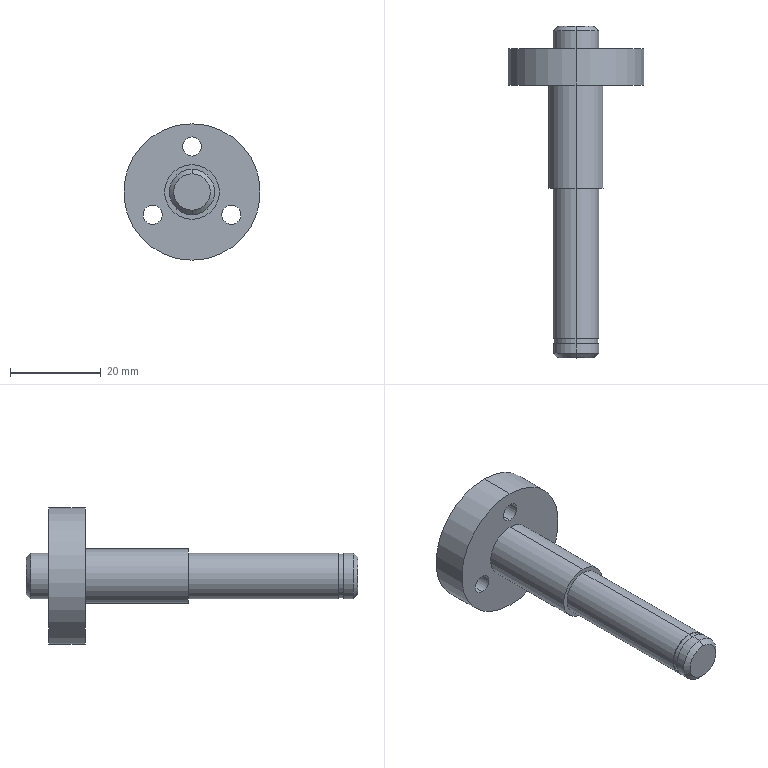Part | STEP file | 0229_207_Pin | 1 solid | 29 faces | box 30 x 73 x 30 mm | volume 11176 mm3 | cylinder 18 | plane 7 | cone 4 | commonest cylinder face diameters 4.2 x6 10 x6 9.6 x2 12 x2 30 x2